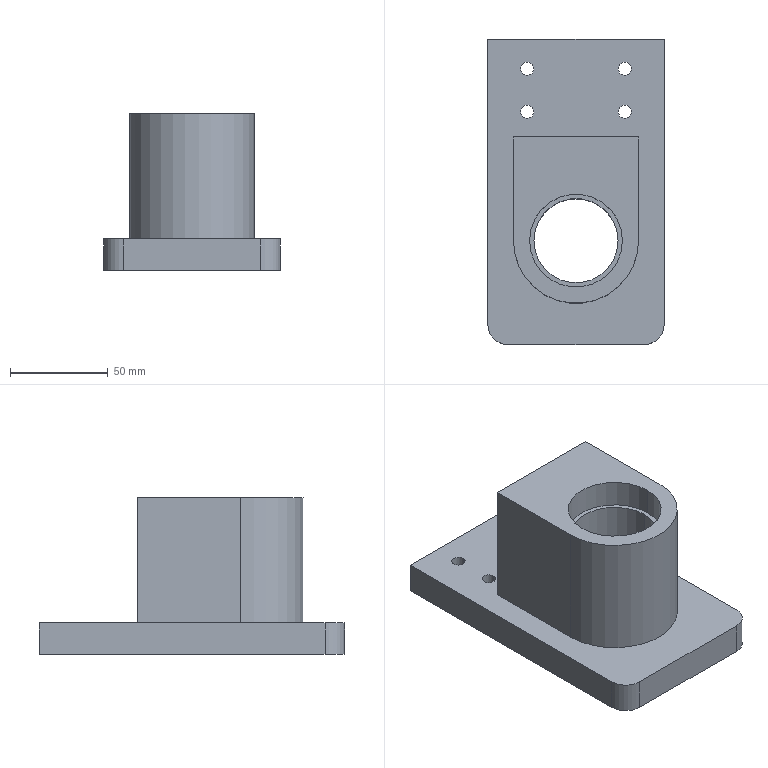NC program | NX | posted with a generic post | part box 90 x 156 x 80 mm
Lines 8430 to 8711 of 8711:
(PLANAR_MILL_3 , TOOL : D16-48-D16-100-3T-FINISH)
N16846 T02 M6
N16848 G53
N16850 G17 G0 G90 X-94. Y0. S2000 M3
N16852 G43 Z30. H2
N16854 Z-61.
N16856 G94 G1 Z-64. F600.
N16858 X-78.
N16860 Y45.
N16862 X68.
N16864 G2 X78. Y35. R10.
N16866 G1 Y-35.
N16868 G2 X68. Y-45. R10.
N16870 G1 X47.824
N16872 Y-35.4
N16874 G3 X47.824 Y35.4 R42.12
N16876 G1 X68.
N16878 G2 X68.4 Y35. R0.4
N16880 G1 Y-35.
N16882 G2 X68. Y-35.4 R0.4
N16884 G1 X47.824
N16886 Y-45.
N16888 X-78.
N16890 Y0.
N16892 X-68.4
N16894 Y35.4
N16896 X-37.532
N16898 G3 X-38.12 Y32. R10.12
N16900 G1 Y-32.
N16902 G3 X-37.532 Y-35.4 R10.12
N16904 G1 X-35.723 Y-34.755
N16906 G2 X-36.2 Y-32. R8.2
N16908 G1 Y32.
N16910 G2 X-28. Y40.2 R8.2
N16912 G1 X25.
N16914 G2 X65.2 Y0. R40.2
N16916 X25. Y-40.2 R40.2
N16918 G1 X-28.
N16920 G2 X-35.723 Y-34.755 R8.2
N16922 G1 X-37.532 Y-35.4
N16924 X-68.4
N16926 Y0.
N16928 X-58.8
N16930 Y25.8
N16932 X-47.72
N16934 Y-25.8
N16936 X-58.8
N16938 Y0.
N16940 X-94.
N16942 Z-61.
N16944 G0 Z30.
(PLANAR_MILL_1 , TOOL : D16-48-D16-100-3T-FINISH)
N16946 X27. Y-42.1
N16948 Z-19.333
N16950 G1 Z-21.333
N16952 G3 X25. Y-40.1 R2.
N16954 G1 X-28.
N16956 G2 X-36.1 Y-32. R8.1
N16958 G1 Y32.
N16960 G2 X-28. Y40.1 R8.1
N16962 G1 X25.
N16964 G2 X65.1 Y0. R40.1
N16966 X25. Y-40.1 R40.1
N16968 G3 X23. Y-42.1 R2.
N16970 G1 X27. Y-42.
N16972 G3 X25. Y-40. R2.
N16974 G1 X-28.
N16976 G2 X-36. Y-32. R8.
N16978 G1 Y32.
N16980 G2 X-28. Y40. R8.
N16982 G1 X25.
N16984 G2 X65. Y0. R40.
N16986 X25. Y-40. R40.
N16988 G3 X23. Y-42. R2.
N16990 G1 Y-42.1
N16992 Z-19.333
N16994 G0 Z30.
N16996 X27.
N16998 Z-40.667
N17000 G1 Z-42.667
N17002 G3 X25. Y-40.1 R2.
N17004 G1 X-28.
N17006 G2 X-36.1 Y-32. R8.1
N17008 G1 Y32.
N17010 G2 X-28. Y40.1 R8.1
N17012 G1 X25.
N17014 G2 X65.1 Y0. R40.1
N17016 X25. Y-40.1 R40.1
N17018 G3 X23. Y-42.1 R2.
N17020 G1 X27. Y-42.
N17022 G3 X25. Y-40. R2.
N17024 G1 X-28.
N17026 G2 X-36. Y-32. R8.
N17028 G1 Y32.
N17030 G2 X-28. Y40. R8.
N17032 G1 X25.
N17034 G2 X65. Y0. R40.
N17036 X25. Y-40. R40.
N17038 G3 X23. Y-42. R2.
N17040 G1 Y-42.1
N17042 Z-40.667
N17044 G0 Z30.
N17046 X27.
N17048 Z-62.
N17050 G1 Z-64.
N17052 G3 X25. Y-40.1 R2.
N17054 G1 X-28.
N17056 G2 X-36.1 Y-32. R8.1
N17058 G1 Y32.
N17060 G2 X-28. Y40.1 R8.1
N17062 G1 X25.
N17064 G2 X65.1 Y0. R40.1
N17066 X25. Y-40.1 R40.1
N17068 G3 X23. Y-42.1 R2.
N17070 G1 X27. Y-42.
N17072 G3 X25. Y-40. R2.
N17074 G1 X-28.
N17076 G2 X-36. Y-32. R8.
N17078 G1 Y32.
N17080 G2 X-28. Y40. R8.
N17082 G1 X25.
N17084 G2 X65. Y0. R40.
N17086 X25. Y-40. R40.
N17088 G3 X23. Y-42. R2.
N17090 G1 Y-42.1
N17092 Z-62.
N17094 G0 Z30.
(PLANAR_MILL_1_COPY , TOOL : D16-48-D16-100-3T-FINISH)
N17096 X-76. Y-55.1
N17098 Z-79.
N17100 G1 Z-81.
N17102 G3 X-78. Y-53.1 R2.
N17104 G2 X-86.1 Y-45. R8.1
N17106 G1 Y45.
N17108 G2 X-78. Y53.1 R8.1
N17110 G1 X68.
N17112 G2 X86.1 Y35. R18.1
N17114 G1 Y-35.
N17116 G2 X68. Y-53.1 R18.1
N17118 G1 X-78.
N17120 G3 X-80. Y-55.1 R2.
N17122 G1 X-76. Y-55.
N17124 G3 X-78. Y-53. R2.
N17126 G2 X-86. Y-45. R8.
N17128 G1 Y45.
N17130 G2 X-78. Y53. R8.
N17132 G1 X68.
N17134 G2 X86. Y35. R18.
N17136 G1 Y-35.
N17138 G2 X68. Y-53. R18.
N17140 G1 X-78.
N17142 G3 X-80. Y-55. R2.
N17144 G1 Z-79.
N17146 G0 Z30.
(PLANAR_MILL_2 , TOOL : D16-48-D16-100-3T-FINISH)
N17148 X23. Y-13.503
N17150 Z-12.
N17152 G1 Z-14.
N17154 Y-13.65
N17156 G3 X25. Y-15.65 R2.
N17158 X40.65 Y0. R15.65
N17160 X25. Y-15.65 R-15.65
N17162 X27. Y-13.65 R2.
N17164 G1 X23. Y-13.75
N17166 G3 X25. Y-15.75 R2.
N17168 X40.75 Y0. R15.75
N17170 X25. Y-15.75 R-15.75
N17172 X27. Y-13.75 R2.
N17174 G1 Y-13.604
N17176 Z-12.
N17178 G0 Z30.
(PLANAR_MILL_2_COPY , TOOL : D16-48-D16-100-3T-FINISH)
N17180 Y11.223
N17182 Z-30.
N17184 G1 Z-32.
N17186 Y11.4
N17188 G3 X25. Y13.4 R2.
N17190 X11.6 Y0. R13.4
N17192 X25. Y13.4 R-13.4
N17194 X23. Y11.4 R2.
N17196 G1 X27. Y11.5
N17198 G3 X25. Y13.5 R2.
N17200 X11.5 Y0. R13.5
N17202 X25. Y13.5 R-13.5
N17204 X23. Y11.5 R2.
N17206 G1 Y11.325
N17208 Z-30.
N17210 G0 Z30.
N17212 X27. Y11.223
N17214 Z-48.
N17216 G1 Z-50.
N17218 Y11.4
N17220 G3 X25. Y13.4 R2.
N17222 X11.6 Y0. R13.4
N17224 X25. Y13.4 R-13.4
N17226 X23. Y11.4 R2.
N17228 G1 X27. Y11.5
N17230 G3 X25. Y13.5 R2.
N17232 X11.5 Y0. R13.5
N17234 X25. Y13.5 R-13.5
N17236 X23. Y11.5 R2.
N17238 G1 Y11.325
N17240 Z-48.
N17242 G0 Z30.
N17244 X27. Y11.223
N17246 Z-66.
N17248 G1 Z-68.
N17250 Y11.4
N17252 G3 X25. Y13.4 R2.
N17254 X11.6 Y0. R13.4
N17256 X25. Y13.4 R-13.4
N17258 X23. Y11.4 R2.
N17260 G1 X27. Y11.5
N17262 G3 X25. Y13.5 R2.
N17264 X11.5 Y0. R13.5
N17266 X25. Y13.5 R-13.5
N17268 X23. Y11.5 R2.
N17270 G1 Y11.325
N17272 Z-66.
N17274 G0 Z30.
N17276 M5
(PLANAR_MILL_4 , TOOL : 倒角D10-90度)
N17278 T04 M6
N17280 G53
N17282 G17 G0 G90 X23. Y-19.648 S3000 M3
N17284 G43 Z30. H4
N17286 Z0.
N17288 G94 G1 Z-2. F800.
N17290 Y-19.75
N17292 G3 X25. Y-21.75 R2.
N17294 X46.75 Y0. R21.75
N17296 X25. Y-21.75 R-21.75
N17298 X27. Y-19.75 R2.
N17300 G1 Y-19.648
N17302 Z0.
N17304 G0 Z30.
(PLANAR_MILL_4_COPY , TOOL : 倒角D10-90度)
N17306 X-32. Y-2.
N17308 Z0.
N17310 G1 Z-2.
N17312 G3 X-30. Y0. R2.
N17314 G1 Y32.
N17316 G2 X-28. Y34. R2.
N17318 G1 X25.
N17320 G2 X59. Y0. R34.
N17322 X25. Y-34. R34.
N17324 G1 X-28.
N17326 G2 X-30. Y-32. R2.
N17328 G1 Y0.
N17330 G3 X-32. Y2. R2.
N17332 G1 Z0.
N17334 G0 Z30.
(PLANAR_MILL_4_COPY_1 , TOOL : 倒角D10-90度)
N17336 X27. Y15.37
N17338 Z-16.
N17340 G1 Z-18.
N17342 Y15.5
N17344 G3 X25. Y17.5 R2.
N17346 X7.5 Y0. R17.5
N17348 X25. Y17.5 R-17.5
N17350 X23. Y15.5 R2.
N17352 G1 Y15.37
N17354 Z-16.
N17356 G0 Z30.
N17358 M5
N17360 M2